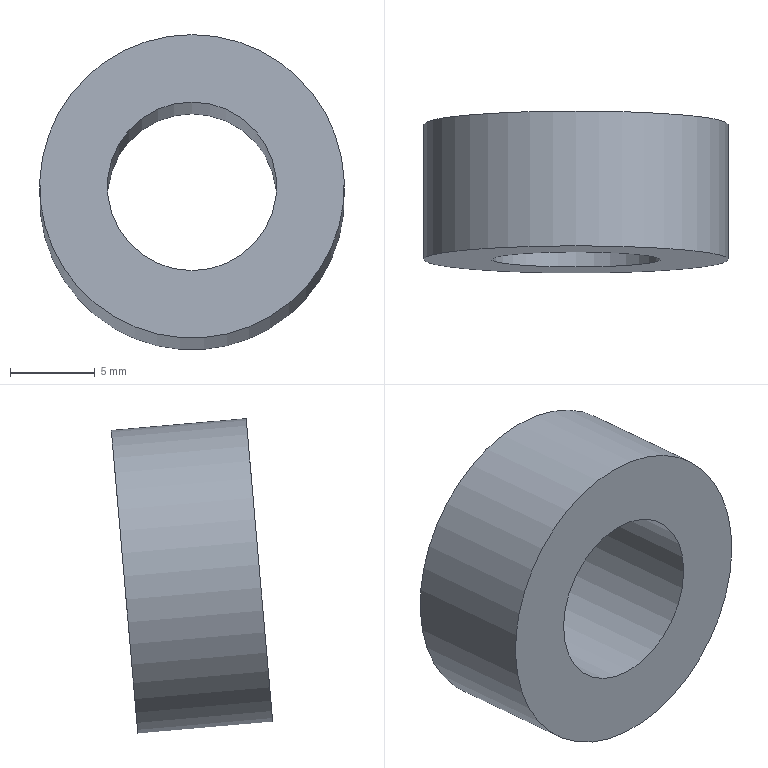Part | NX | features solid 2 | 1 solid | 4 faces | box 18 x 9.538 x 18.629 mm | volume 1407 mm3 | cylinder 2 | plane 2 | commonest cylinder face diameters 10 x1 18 x1
STEP:
#1=CARTESIAN_POINT('',(280.775,-72.524,-39.563));
#2=VERTEX_POINT('',#1);
#3=CARTESIAN_POINT('',(280.775,-73.309,-48.529));
#4=DIRECTION('',(0.,0.9962,-0.08716));
#5=DIRECTION('',(0.,0.08716,0.9962));
#6=AXIS2_PLACEMENT_3D('',#3,#4,#5);
#7=CIRCLE('',#6,9.);
#8=EDGE_CURVE('',#2,#2,#7,.F.);
#9=ORIENTED_EDGE('',*,*,#8,.T.);
#10=EDGE_LOOP('',(#9));
#11=FACE_BOUND('',#10,.T.);
#12=CARTESIAN_POINT('',(280.775,-80.494,-38.866));
#13=VERTEX_POINT('',#12);
#14=CARTESIAN_POINT('',(280.775,-81.278,-47.832));
#15=DIRECTION('',(0.,0.9962,-0.08716));
#16=DIRECTION('',(0.,0.08716,0.9962));
#17=AXIS2_PLACEMENT_3D('',#14,#15,#16);
#18=CIRCLE('',#17,9.);
#19=EDGE_CURVE('',#13,#13,#18,.F.);
#20=ORIENTED_EDGE('',*,*,#19,.F.);
#21=EDGE_LOOP('',(#20));
#22=FACE_BOUND('',#21,.T.);
#23=CARTESIAN_POINT('',(280.775,-73.309,-48.529));
#24=DIRECTION('',(0.,-0.9962,0.08716));
#25=DIRECTION('',(0.,-0.08716,-0.9962));
#26=AXIS2_PLACEMENT_3D('',#23,#24,#25);
#27=CYLINDRICAL_SURFACE('',#26,9.);
#28=ADVANCED_FACE('',(#11,#22),#27,.T.);
#29=CARTESIAN_POINT('',(280.775,-73.745,-53.51));
#30=VERTEX_POINT('',#29);
#31=CARTESIAN_POINT('',(280.775,-73.309,-48.529));
#32=DIRECTION('',(0.,-0.9962,0.08716));
#33=DIRECTION('',(0.,-0.08716,-0.9962));
#34=AXIS2_PLACEMENT_3D('',#31,#32,#33);
#35=CIRCLE('',#34,5.);
#36=EDGE_CURVE('',#30,#30,#35,.T.);
#37=ORIENTED_EDGE('',*,*,#36,.T.);
#38=EDGE_LOOP('',(#37));
#39=FACE_BOUND('',#38,.T.);
#40=ORIENTED_EDGE('',*,*,#8,.F.);
#41=EDGE_LOOP('',(#40));
#42=FACE_BOUND('',#41,.T.);
#43=CARTESIAN_POINT('',(280.775,-73.309,-48.529));
#44=DIRECTION('',(0.,0.9962,-0.08716));
#45=DIRECTION('',(-1.,0.,0.));
#46=AXIS2_PLACEMENT_3D('',#43,#44,#45);
#47=PLANE('',#46);
#48=ADVANCED_FACE('',(#39,#42),#47,.T.);
#49=CARTESIAN_POINT('',(280.775,-80.843,-42.851));
#50=VERTEX_POINT('',#49);
#51=CARTESIAN_POINT('',(280.775,-81.278,-47.832));
#52=DIRECTION('',(0.,0.9962,-0.08716));
#53=DIRECTION('',(0.,0.08716,0.9962));
#54=AXIS2_PLACEMENT_3D('',#51,#52,#53);
#55=CIRCLE('',#54,5.);
#56=EDGE_CURVE('',#50,#50,#55,.T.);
#57=ORIENTED_EDGE('',*,*,#56,.T.);
#58=EDGE_LOOP('',(#57));
#59=FACE_BOUND('',#58,.T.);
#60=ORIENTED_EDGE('',*,*,#19,.T.);
#61=EDGE_LOOP('',(#60));
#62=FACE_BOUND('',#61,.T.);
#63=CARTESIAN_POINT('',(280.775,-81.278,-47.832));
#64=DIRECTION('',(0.,0.9962,-0.08716));
#65=DIRECTION('',(-1.,0.,0.));
#66=AXIS2_PLACEMENT_3D('',#63,#64,#65);
#67=PLANE('',#66);
#68=ADVANCED_FACE('',(#59,#62),#67,.F.);
#69=ORIENTED_EDGE('',*,*,#36,.F.);
#70=EDGE_LOOP('',(#69));
#71=FACE_BOUND('',#70,.T.);
#72=ORIENTED_EDGE('',*,*,#56,.F.);
#73=EDGE_LOOP('',(#72));
#74=FACE_BOUND('',#73,.T.);
#75=CARTESIAN_POINT('',(280.775,-73.309,-48.529));
#76=DIRECTION('',(0.,-0.9962,0.08716));
#77=DIRECTION('',(0.,-0.08716,-0.9962));
#78=AXIS2_PLACEMENT_3D('',#75,#76,#77);
#79=CYLINDRICAL_SURFACE('',#78,5.);
#80=ADVANCED_FACE('',(#71,#74),#79,.F.);
#81=CLOSED_SHELL('',(#28,#48,#68,#80));
#82=MANIFOLD_SOLID_BREP('',#81);
#83=(LENGTH_UNIT()NAMED_UNIT(*)SI_UNIT(.MILLI.,.METRE.));
#84=UNCERTAINTY_MEASURE_WITH_UNIT(LENGTH_MEASURE(0.00001),#83,'','');
#85=(NAMED_UNIT(*)PLANE_ANGLE_UNIT()SI_UNIT($,.RADIAN.));
#86=(NAMED_UNIT(*)SI_UNIT($,.STERADIAN.)SOLID_ANGLE_UNIT());
#87=(GEOMETRIC_REPRESENTATION_CONTEXT(3)GLOBAL_UNCERTAINTY_ASSIGNED_CONTEXT((#84))GLOBAL_UNIT_ASSIGNED_CONTEXT((#83,#85,#86))REPRESENTATION_CONTEXT('',''));
#88=ADVANCED_BREP_SHAPE_REPRESENTATION('',(#82),#87);